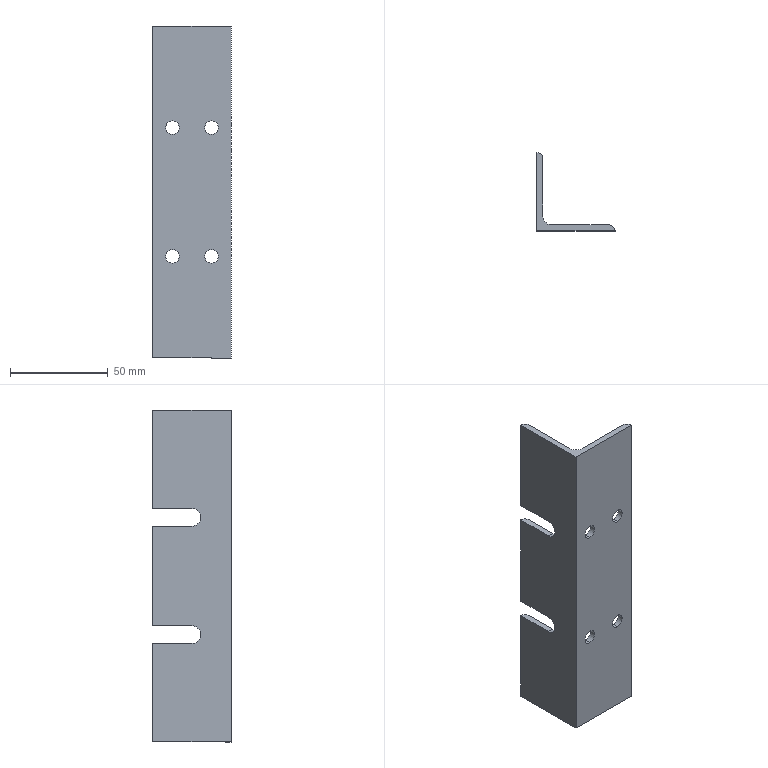Part | SolidWorks | features BaseBody 1 | 1 solid | 25 faces | box 40 x 40 x 170 mm | volume 37654 mm3 | cylinder 15 | plane 10 | commonest cylinder face diameters 7 x8 6 x4 9 x3
STEP:
#1=CARTESIAN_POINT('',(30.,3.,-29.45));
#2=VERTEX_POINT('',#1);
#3=CARTESIAN_POINT('',(30.,0.,-29.45));
#4=VERTEX_POINT('',#3);
#5=CARTESIAN_POINT('',(30.,10.,-29.45));
#6=DIRECTION('',(0.,-1.,0.));
#7=VECTOR('',#6,1000.);
#8=LINE('',#5,#7);
#9=EDGE_CURVE('',#2,#4,#8,.T.);
#10=ORIENTED_EDGE('',*,*,#9,.F.);
#11=CARTESIAN_POINT('',(30.,3.,-36.45));
#12=VERTEX_POINT('',#11);
#13=CARTESIAN_POINT('',(30.,3.,-32.95));
#14=DIRECTION('',(0.,-1.,0.));
#15=DIRECTION('',(0.,0.,-1.));
#16=AXIS2_PLACEMENT_3D('',#13,#14,#15);
#17=CIRCLE('',#16,3.5);
#18=EDGE_CURVE('',#12,#2,#17,.T.);
#19=ORIENTED_EDGE('',*,*,#18,.F.);
#20=CARTESIAN_POINT('',(30.,0.,-36.45));
#21=VERTEX_POINT('',#20);
#22=CARTESIAN_POINT('',(30.,10.,-36.45));
#23=DIRECTION('',(0.,-1.,0.));
#24=VECTOR('',#23,1000.);
#25=LINE('',#22,#24);
#26=EDGE_CURVE('',#12,#21,#25,.T.);
#27=ORIENTED_EDGE('',*,*,#26,.T.);
#28=CARTESIAN_POINT('',(30.,0.,-32.95));
#29=DIRECTION('',(0.,-1.,0.));
#30=DIRECTION('',(0.,0.,1.));
#31=AXIS2_PLACEMENT_3D('',#28,#29,#30);
#32=CIRCLE('',#31,3.5);
#33=EDGE_CURVE('',#21,#4,#32,.T.);
#34=ORIENTED_EDGE('',*,*,#33,.T.);
#35=EDGE_LOOP('',(#10,#19,#27,#34));
#36=FACE_OUTER_BOUND('',#35,.T.);
#37=CARTESIAN_POINT('',(30.,10.,-32.95));
#38=DIRECTION('',(0.,-1.,0.));
#39=DIRECTION('',(0.,0.,-1.));
#40=AXIS2_PLACEMENT_3D('',#37,#38,#39);
#41=CYLINDRICAL_SURFACE('',#40,3.5);
#42=ADVANCED_FACE('',(#36),#41,.F.);
#43=CARTESIAN_POINT('',(30.,3.,36.45));
#44=VERTEX_POINT('',#43);
#45=CARTESIAN_POINT('',(30.,0.,36.45));
#46=VERTEX_POINT('',#45);
#47=CARTESIAN_POINT('',(30.,10.,36.45));
#48=DIRECTION('',(0.,-1.,0.));
#49=VECTOR('',#48,1000.);
#50=LINE('',#47,#49);
#51=EDGE_CURVE('',#44,#46,#50,.T.);
#52=ORIENTED_EDGE('',*,*,#51,.F.);
#53=CARTESIAN_POINT('',(30.,3.,29.45));
#54=VERTEX_POINT('',#53);
#55=CARTESIAN_POINT('',(30.,3.,32.95));
#56=DIRECTION('',(0.,-1.,0.));
#57=DIRECTION('',(0.,0.,-1.));
#58=AXIS2_PLACEMENT_3D('',#55,#56,#57);
#59=CIRCLE('',#58,3.5);
#60=EDGE_CURVE('',#54,#44,#59,.T.);
#61=ORIENTED_EDGE('',*,*,#60,.F.);
#62=CARTESIAN_POINT('',(30.,0.,29.45));
#63=VERTEX_POINT('',#62);
#64=CARTESIAN_POINT('',(30.,10.,29.45));
#65=DIRECTION('',(0.,-1.,0.));
#66=VECTOR('',#65,1000.);
#67=LINE('',#64,#66);
#68=EDGE_CURVE('',#54,#63,#67,.T.);
#69=ORIENTED_EDGE('',*,*,#68,.T.);
#70=CARTESIAN_POINT('',(30.,0.,32.95));
#71=DIRECTION('',(0.,-1.,0.));
#72=DIRECTION('',(0.,0.,-1.));
#73=AXIS2_PLACEMENT_3D('',#70,#71,#72);
#74=CIRCLE('',#73,3.5);
#75=EDGE_CURVE('',#63,#46,#74,.T.);
#76=ORIENTED_EDGE('',*,*,#75,.T.);
#77=EDGE_LOOP('',(#52,#61,#69,#76));
#78=FACE_OUTER_BOUND('',#77,.T.);
#79=CARTESIAN_POINT('',(30.,10.,32.95));
#80=DIRECTION('',(0.,-1.,0.));
#81=DIRECTION('',(0.,0.,-1.));
#82=AXIS2_PLACEMENT_3D('',#79,#80,#81);
#83=CYLINDRICAL_SURFACE('',#82,3.5);
#84=ADVANCED_FACE('',(#78),#83,.F.);
#85=CARTESIAN_POINT('',(10.,3.,-29.45));
#86=VERTEX_POINT('',#85);
#87=CARTESIAN_POINT('',(10.,0.,-29.45));
#88=VERTEX_POINT('',#87);
#89=CARTESIAN_POINT('',(10.,10.,-29.45));
#90=DIRECTION('',(0.,-1.,0.));
#91=VECTOR('',#90,1000.);
#92=LINE('',#89,#91);
#93=EDGE_CURVE('',#86,#88,#92,.T.);
#94=ORIENTED_EDGE('',*,*,#93,.F.);
#95=CARTESIAN_POINT('',(10.,3.,-36.45));
#96=VERTEX_POINT('',#95);
#97=CARTESIAN_POINT('',(10.,3.,-32.95));
#98=DIRECTION('',(0.,-1.,0.));
#99=DIRECTION('',(0.,0.,-1.));
#100=AXIS2_PLACEMENT_3D('',#97,#98,#99);
#101=CIRCLE('',#100,3.5);
#102=EDGE_CURVE('',#96,#86,#101,.T.);
#103=ORIENTED_EDGE('',*,*,#102,.F.);
#104=CARTESIAN_POINT('',(10.,0.,-36.45));
#105=VERTEX_POINT('',#104);
#106=CARTESIAN_POINT('',(10.,10.,-36.45));
#107=DIRECTION('',(0.,-1.,0.));
#108=VECTOR('',#107,1000.);
#109=LINE('',#106,#108);
#110=EDGE_CURVE('',#96,#105,#109,.T.);
#111=ORIENTED_EDGE('',*,*,#110,.T.);
#112=CARTESIAN_POINT('',(10.,0.,-32.95));
#113=DIRECTION('',(0.,-1.,0.));
#114=DIRECTION('',(0.,0.,1.));
#115=AXIS2_PLACEMENT_3D('',#112,#113,#114);
#116=CIRCLE('',#115,3.5);
#117=EDGE_CURVE('',#105,#88,#116,.T.);
#118=ORIENTED_EDGE('',*,*,#117,.T.);
#119=EDGE_LOOP('',(#94,#103,#111,#118));
#120=FACE_OUTER_BOUND('',#119,.T.);
#121=CARTESIAN_POINT('',(10.,10.,-32.95));
#122=DIRECTION('',(0.,-1.,0.));
#123=DIRECTION('',(0.,0.,-1.));
#124=AXIS2_PLACEMENT_3D('',#121,#122,#123);
#125=CYLINDRICAL_SURFACE('',#124,3.5);
#126=ADVANCED_FACE('',(#120),#125,.F.);
#127=CARTESIAN_POINT('',(10.,3.,36.45));
#128=VERTEX_POINT('',#127);
#129=CARTESIAN_POINT('',(10.,0.,36.45));
#130=VERTEX_POINT('',#129);
#131=CARTESIAN_POINT('',(10.,10.,36.45));
#132=DIRECTION('',(0.,-1.,0.));
#133=VECTOR('',#132,1000.);
#134=LINE('',#131,#133);
#135=EDGE_CURVE('',#128,#130,#134,.T.);
#136=ORIENTED_EDGE('',*,*,#135,.F.);
#137=CARTESIAN_POINT('',(10.,3.,29.45));
#138=VERTEX_POINT('',#137);
#139=CARTESIAN_POINT('',(10.,3.,32.95));
#140=DIRECTION('',(0.,-1.,0.));
#141=DIRECTION('',(0.,0.,-1.));
#142=AXIS2_PLACEMENT_3D('',#139,#140,#141);
#143=CIRCLE('',#142,3.5);
#144=EDGE_CURVE('',#138,#128,#143,.T.);
#145=ORIENTED_EDGE('',*,*,#144,.F.);
#146=CARTESIAN_POINT('',(10.,0.,29.45));
#147=VERTEX_POINT('',#146);
#148=CARTESIAN_POINT('',(10.,10.,29.45));
#149=DIRECTION('',(0.,-1.,0.));
#150=VECTOR('',#149,1000.);
#151=LINE('',#148,#150);
#152=EDGE_CURVE('',#138,#147,#151,.T.);
#153=ORIENTED_EDGE('',*,*,#152,.T.);
#154=CARTESIAN_POINT('',(10.,0.,32.95));
#155=DIRECTION('',(0.,-1.,0.));
#156=DIRECTION('',(0.,0.,-1.));
#157=AXIS2_PLACEMENT_3D('',#154,#155,#156);
#158=CIRCLE('',#157,3.5);
#159=EDGE_CURVE('',#147,#130,#158,.T.);
#160=ORIENTED_EDGE('',*,*,#159,.T.);
#161=EDGE_LOOP('',(#136,#145,#153,#160));
#162=FACE_OUTER_BOUND('',#161,.T.);
#163=CARTESIAN_POINT('',(10.,10.,32.95));
#164=DIRECTION('',(0.,-1.,0.));
#165=DIRECTION('',(0.,0.,-1.));
#166=AXIS2_PLACEMENT_3D('',#163,#164,#165);
#167=CYLINDRICAL_SURFACE('',#166,3.5);
#168=ADVANCED_FACE('',(#162),#167,.F.);
#169=CARTESIAN_POINT('',(3.,37.,25.5));
#170=VERTEX_POINT('',#169);
#171=CARTESIAN_POINT('',(0.,40.,25.5));
#172=VERTEX_POINT('',#171);
#173=CARTESIAN_POINT('',(0.,37.,25.5));
#174=DIRECTION('',(0.,0.,1.));
#175=DIRECTION('',(0.,1.,0.));
#176=AXIS2_PLACEMENT_3D('',#173,#174,#175);
#177=CIRCLE('',#176,3.);
#178=EDGE_CURVE('',#170,#172,#177,.T.);
#179=ORIENTED_EDGE('',*,*,#178,.T.);
#180=CARTESIAN_POINT('',(0.,20.,25.5));
#181=VERTEX_POINT('',#180);
#182=CARTESIAN_POINT('',(0.,40.,25.5));
#183=DIRECTION('',(0.,-1.,0.));
#184=VECTOR('',#183,1000.);
#185=LINE('',#182,#184);
#186=EDGE_CURVE('',#172,#181,#185,.T.);
#187=ORIENTED_EDGE('',*,*,#186,.T.);
#188=CARTESIAN_POINT('',(3.,20.,25.5));
#189=VERTEX_POINT('',#188);
#190=CARTESIAN_POINT('',(10.,20.,25.5));
#191=DIRECTION('',(-1.,0.,0.));
#192=VECTOR('',#191,1000.);
#193=LINE('',#190,#192);
#194=EDGE_CURVE('',#189,#181,#193,.T.);
#195=ORIENTED_EDGE('',*,*,#194,.F.);
#196=CARTESIAN_POINT('',(3.,40.,25.5));
#197=DIRECTION('',(0.,-1.,0.));
#198=VECTOR('',#197,1000.);
#199=LINE('',#196,#198);
#200=EDGE_CURVE('',#170,#189,#199,.T.);
#201=ORIENTED_EDGE('',*,*,#200,.F.);
#202=EDGE_LOOP('',(#179,#187,#195,#201));
#203=FACE_OUTER_BOUND('',#202,.T.);
#204=CARTESIAN_POINT('',(10.,40.,25.5));
#205=DIRECTION('',(0.,0.,-1.));
#206=DIRECTION('',(0.,-1.,0.));
#207=AXIS2_PLACEMENT_3D('',#204,#205,#206);
#208=PLANE('',#207);
#209=ADVANCED_FACE('',(#203),#208,.F.);
#210=CARTESIAN_POINT('',(3.,20.,34.5));
#211=VERTEX_POINT('',#210);
#212=CARTESIAN_POINT('',(0.,20.,34.5));
#213=VERTEX_POINT('',#212);
#214=CARTESIAN_POINT('',(10.,20.,34.5));
#215=DIRECTION('',(-1.,0.,0.));
#216=VECTOR('',#215,1000.);
#217=LINE('',#214,#216);
#218=EDGE_CURVE('',#211,#213,#217,.T.);
#219=ORIENTED_EDGE('',*,*,#218,.T.);
#220=CARTESIAN_POINT('',(0.,40.,34.5));
#221=VERTEX_POINT('',#220);
#222=CARTESIAN_POINT('',(0.,40.,34.5));
#223=DIRECTION('',(0.,1.,0.));
#224=VECTOR('',#223,1000.);
#225=LINE('',#222,#224);
#226=EDGE_CURVE('',#213,#221,#225,.T.);
#227=ORIENTED_EDGE('',*,*,#226,.T.);
#228=CARTESIAN_POINT('',(3.,37.,34.5));
#229=VERTEX_POINT('',#228);
#230=CARTESIAN_POINT('',(0.,37.,34.5));
#231=DIRECTION('',(0.,0.,-1.));
#232=DIRECTION('',(0.,-1.,0.));
#233=AXIS2_PLACEMENT_3D('',#230,#231,#232);
#234=CIRCLE('',#233,3.);
#235=EDGE_CURVE('',#221,#229,#234,.T.);
#236=ORIENTED_EDGE('',*,*,#235,.T.);
#237=CARTESIAN_POINT('',(3.,40.,34.5));
#238=DIRECTION('',(0.,1.,0.));
#239=VECTOR('',#238,1000.);
#240=LINE('',#237,#239);
#241=EDGE_CURVE('',#211,#229,#240,.T.);
#242=ORIENTED_EDGE('',*,*,#241,.F.);
#243=EDGE_LOOP('',(#219,#227,#236,#242));
#244=FACE_OUTER_BOUND('',#243,.T.);
#245=CARTESIAN_POINT('',(10.,40.,34.5));
#246=DIRECTION('',(0.,0.,1.));
#247=DIRECTION('',(0.,-1.,0.));
#248=AXIS2_PLACEMENT_3D('',#245,#246,#247);
#249=PLANE('',#248);
#250=ADVANCED_FACE('',(#244),#249,.F.);
#251=ORIENTED_EDGE('',*,*,#194,.T.);
#252=CARTESIAN_POINT('',(0.,20.,30.));
#253=DIRECTION('',(-1.,0.,0.));
#254=DIRECTION('',(0.,0.,1.));
#255=AXIS2_PLACEMENT_3D('',#252,#253,#254);
#256=CIRCLE('',#255,4.5);
#257=EDGE_CURVE('',#181,#213,#256,.T.);
#258=ORIENTED_EDGE('',*,*,#257,.T.);
#259=ORIENTED_EDGE('',*,*,#218,.F.);
#260=CARTESIAN_POINT('',(3.,20.,30.));
#261=DIRECTION('',(-1.,0.,0.));
#262=DIRECTION('',(0.,-1.,0.));
#263=AXIS2_PLACEMENT_3D('',#260,#261,#262);
#264=CIRCLE('',#263,4.5);
#265=EDGE_CURVE('',#189,#211,#264,.T.);
#266=ORIENTED_EDGE('',*,*,#265,.F.);
#267=EDGE_LOOP('',(#251,#258,#259,#266));
#268=FACE_OUTER_BOUND('',#267,.T.);
#269=CARTESIAN_POINT('',(10.,20.,30.));
#270=DIRECTION('',(-1.,0.,0.));
#271=DIRECTION('',(0.,0.,1.));
#272=AXIS2_PLACEMENT_3D('',#269,#270,#271);
#273=CYLINDRICAL_SURFACE('',#272,4.5);
#274=ADVANCED_FACE('',(#268),#273,.F.);
#275=CARTESIAN_POINT('',(3.,37.,-34.5));
#276=VERTEX_POINT('',#275);
#277=CARTESIAN_POINT('',(0.,40.,-34.5));
#278=VERTEX_POINT('',#277);
#279=CARTESIAN_POINT('',(0.,37.,-34.5));
#280=DIRECTION('',(0.,0.,1.));
#281=DIRECTION('',(0.,1.,0.));
#282=AXIS2_PLACEMENT_3D('',#279,#280,#281);
#283=CIRCLE('',#282,3.);
#284=EDGE_CURVE('',#276,#278,#283,.T.);
#285=ORIENTED_EDGE('',*,*,#284,.T.);
#286=CARTESIAN_POINT('',(0.,20.,-34.5));
#287=VERTEX_POINT('',#286);
#288=CARTESIAN_POINT('',(0.,40.,-34.5));
#289=DIRECTION('',(0.,-1.,0.));
#290=VECTOR('',#289,1000.);
#291=LINE('',#288,#290);
#292=EDGE_CURVE('',#278,#287,#291,.T.);
#293=ORIENTED_EDGE('',*,*,#292,.T.);
#294=CARTESIAN_POINT('',(3.,20.,-34.5));
#295=VERTEX_POINT('',#294);
#296=CARTESIAN_POINT('',(10.,20.,-34.5));
#297=DIRECTION('',(-1.,0.,0.));
#298=VECTOR('',#297,1000.);
#299=LINE('',#296,#298);
#300=EDGE_CURVE('',#295,#287,#299,.T.);
#301=ORIENTED_EDGE('',*,*,#300,.F.);
#302=CARTESIAN_POINT('',(3.,40.,-34.5));
#303=DIRECTION('',(0.,-1.,0.));
#304=VECTOR('',#303,1000.);
#305=LINE('',#302,#304);
#306=EDGE_CURVE('',#276,#295,#305,.T.);
#307=ORIENTED_EDGE('',*,*,#306,.F.);
#308=EDGE_LOOP('',(#285,#293,#301,#307));
#309=FACE_OUTER_BOUND('',#308,.T.);
#310=CARTESIAN_POINT('',(10.,40.,-34.5));
#311=DIRECTION('',(0.,0.,-1.));
#312=DIRECTION('',(0.,-1.,0.));
#313=AXIS2_PLACEMENT_3D('',#310,#311,#312);
#314=PLANE('',#313);
#315=ADVANCED_FACE('',(#309),#314,.F.);
#316=CARTESIAN_POINT('',(3.,20.,-25.5));
#317=VERTEX_POINT('',#316);
#318=CARTESIAN_POINT('',(0.,20.,-25.5));
#319=VERTEX_POINT('',#318);
#320=CARTESIAN_POINT('',(10.,20.,-25.5));
#321=DIRECTION('',(-1.,0.,0.));
#322=VECTOR('',#321,1000.);
#323=LINE('',#320,#322);
#324=EDGE_CURVE('',#317,#319,#323,.T.);
#325=ORIENTED_EDGE('',*,*,#324,.T.);
#326=CARTESIAN_POINT('',(0.,40.,-25.5));
#327=VERTEX_POINT('',#326);
#328=CARTESIAN_POINT('',(0.,40.,-25.5));
#329=DIRECTION('',(0.,1.,0.));
#330=VECTOR('',#329,1000.);
#331=LINE('',#328,#330);
#332=EDGE_CURVE('',#319,#327,#331,.T.);
#333=ORIENTED_EDGE('',*,*,#332,.T.);
#334=CARTESIAN_POINT('',(3.,37.,-25.5));
#335=VERTEX_POINT('',#334);
#336=CARTESIAN_POINT('',(0.,37.,-25.5));
#337=DIRECTION('',(0.,0.,-1.));
#338=DIRECTION('',(1.,0.,0.));
#339=AXIS2_PLACEMENT_3D('',#336,#337,#338);
#340=CIRCLE('',#339,3.);
#341=EDGE_CURVE('',#327,#335,#340,.T.);
#342=ORIENTED_EDGE('',*,*,#341,.T.);
#343=CARTESIAN_POINT('',(3.,40.,-25.5));
#344=DIRECTION('',(0.,1.,0.));
#345=VECTOR('',#344,1000.);
#346=LINE('',#343,#345);
#347=EDGE_CURVE('',#317,#335,#346,.T.);
#348=ORIENTED_EDGE('',*,*,#347,.F.);
#349=EDGE_LOOP('',(#325,#333,#342,#348));
#350=FACE_OUTER_BOUND('',#349,.T.);
#351=CARTESIAN_POINT('',(10.,40.,-25.5));
#352=DIRECTION('',(0.,0.,1.));
#353=DIRECTION('',(1.,0.,0.));
#354=AXIS2_PLACEMENT_3D('',#351,#352,#353);
#355=PLANE('',#354);
#356=ADVANCED_FACE('',(#350),#355,.F.);
#357=ORIENTED_EDGE('',*,*,#300,.T.);
#358=CARTESIAN_POINT('',(0.,20.,-30.));
#359=DIRECTION('',(-1.,0.,0.));
#360=DIRECTION('',(0.,0.,-1.));
#361=AXIS2_PLACEMENT_3D('',#358,#359,#360);
#362=CIRCLE('',#361,4.5);
#363=EDGE_CURVE('',#287,#319,#362,.T.);
#364=ORIENTED_EDGE('',*,*,#363,.T.);
#365=ORIENTED_EDGE('',*,*,#324,.F.);
#366=CARTESIAN_POINT('',(3.,20.,-30.));
#367=DIRECTION('',(-1.,0.,0.));
#368=DIRECTION('',(0.,-1.,0.));
#369=AXIS2_PLACEMENT_3D('',#366,#367,#368);
#370=CIRCLE('',#369,4.5);
#371=EDGE_CURVE('',#295,#317,#370,.T.);
#372=ORIENTED_EDGE('',*,*,#371,.F.);
#373=EDGE_LOOP('',(#357,#364,#365,#372));
#374=FACE_OUTER_BOUND('',#373,.T.);
#375=CARTESIAN_POINT('',(10.,20.,-30.));
#376=DIRECTION('',(-1.,0.,0.));
#377=DIRECTION('',(0.,0.,1.));
#378=AXIS2_PLACEMENT_3D('',#375,#376,#377);
#379=CYLINDRICAL_SURFACE('',#378,4.5);
#380=ADVANCED_FACE('',(#374),#379,.F.);
#381=ORIENTED_EDGE('',*,*,#284,.F.);
#382=CARTESIAN_POINT('',(3.,37.,-85.));
#383=VERTEX_POINT('',#382);
#384=CARTESIAN_POINT('',(3.,37.,85.));
#385=DIRECTION('',(0.,0.,1.));
#386=VECTOR('',#385,1000.);
#387=LINE('',#384,#386);
#388=EDGE_CURVE('',#383,#276,#387,.T.);
#389=ORIENTED_EDGE('',*,*,#388,.F.);
#390=CARTESIAN_POINT('',(0.,40.,-85.));
#391=VERTEX_POINT('',#390);
#392=CARTESIAN_POINT('',(0.,37.,-85.));
#393=DIRECTION('',(0.,0.,-1.));
#394=DIRECTION('',(-1.,0.,0.));
#395=AXIS2_PLACEMENT_3D('',#392,#393,#394);
#396=CIRCLE('',#395,3.);
#397=EDGE_CURVE('',#391,#383,#396,.T.);
#398=ORIENTED_EDGE('',*,*,#397,.F.);
#399=CARTESIAN_POINT('',(0.,40.,85.));
#400=DIRECTION('',(0.,0.,-1.));
#401=VECTOR('',#400,1000.);
#402=LINE('',#399,#401);
#403=EDGE_CURVE('',#278,#391,#402,.T.);
#404=ORIENTED_EDGE('',*,*,#403,.F.);
#405=EDGE_LOOP('',(#381,#389,#398,#404));
#406=FACE_OUTER_BOUND('',#405,.T.);
#407=CARTESIAN_POINT('',(0.,37.,85.));
#408=DIRECTION('',(0.,0.,-1.));
#409=DIRECTION('',(-1.,0.,0.));
#410=AXIS2_PLACEMENT_3D('',#407,#408,#409);
#411=CYLINDRICAL_SURFACE('',#410,3.);
#412=ADVANCED_FACE('',(#406),#411,.T.);
#413=CARTESIAN_POINT('',(40.,0.,85.));
#414=VERTEX_POINT('',#413);
#415=CARTESIAN_POINT('',(37.,3.,85.));
#416=VERTEX_POINT('',#415);
#417=CARTESIAN_POINT('',(37.,0.,85.));
#418=DIRECTION('',(0.,0.,1.));
#419=DIRECTION('',(-1.,0.,0.));
#420=AXIS2_PLACEMENT_3D('',#417,#418,#419);
#421=CIRCLE('',#420,3.);
#422=EDGE_CURVE('',#414,#416,#421,.T.);
#423=ORIENTED_EDGE('',*,*,#422,.F.);
#424=CARTESIAN_POINT('',(40.,0.,-85.));
#425=VERTEX_POINT('',#424);
#426=CARTESIAN_POINT('',(40.,0.,85.));
#427=DIRECTION('',(0.,0.,-1.));
#428=VECTOR('',#427,1000.);
#429=LINE('',#426,#428);
#430=EDGE_CURVE('',#414,#425,#429,.T.);
#431=ORIENTED_EDGE('',*,*,#430,.T.);
#432=CARTESIAN_POINT('',(37.,3.,-85.));
#433=VERTEX_POINT('',#432);
#434=CARTESIAN_POINT('',(37.,0.,-85.));
#435=DIRECTION('',(0.,0.,-1.));
#436=DIRECTION('',(-1.,0.,0.));
#437=AXIS2_PLACEMENT_3D('',#434,#435,#436);
#438=CIRCLE('',#437,3.);
#439=EDGE_CURVE('',#433,#425,#438,.T.);
#440=ORIENTED_EDGE('',*,*,#439,.F.);
#441=CARTESIAN_POINT('',(37.,3.,85.));
#442=DIRECTION('',(0.,0.,-1.));
#443=VECTOR('',#442,1000.);
#444=LINE('',#441,#443);
#445=EDGE_CURVE('',#416,#433,#444,.T.);
#446=ORIENTED_EDGE('',*,*,#445,.F.);
#447=EDGE_LOOP('',(#423,#431,#440,#446));
#448=FACE_OUTER_BOUND('',#447,.T.);
#449=CARTESIAN_POINT('',(37.,0.,85.));
#450=DIRECTION('',(0.,0.,-1.));
#451=DIRECTION('',(-1.,0.,0.));
#452=AXIS2_PLACEMENT_3D('',#449,#450,#451);
#453=CYLINDRICAL_SURFACE('',#452,3.);
#454=ADVANCED_FACE('',(#448),#453,.T.);
#455=CARTESIAN_POINT('',(7.5,3.,-30.501));
#456=VERTEX_POINT('',#455);
#457=CARTESIAN_POINT('',(7.5,3.,30.501));
#458=VERTEX_POINT('',#457);
#459=CARTESIAN_POINT('',(7.5,3.,85.));
#460=DIRECTION('',(0.,0.,1.));
#461=VECTOR('',#460,1000.);
#462=LINE('',#459,#461);
#463=EDGE_CURVE('',#456,#458,#462,.T.);
#464=ORIENTED_EDGE('',*,*,#463,.F.);
#465=CARTESIAN_POINT('',(7.5,3.,-35.399));
#466=VERTEX_POINT('',#465);
#467=CARTESIAN_POINT('',(7.5,3.,-30.501));
#468=CARTESIAN_POINT('',(7.183,3.,-30.824));
#469=CARTESIAN_POINT('',(6.93,3.033,-31.209));
#470=CARTESIAN_POINT('',(6.673,3.076,-31.84));
#471=CARTESIAN_POINT('',(6.609,3.089,-32.053));
#472=CARTESIAN_POINT('',(6.522,3.107,-32.5));
#473=CARTESIAN_POINT('',(6.5,3.113,-32.726));
#474=CARTESIAN_POINT('',(6.5,3.112,-33.405));
#475=CARTESIAN_POINT('',(6.589,3.09,-33.854));
#476=CARTESIAN_POINT('',(6.932,3.033,-34.694));
#477=CARTESIAN_POINT('',(7.184,3.,-35.077));
#478=CARTESIAN_POINT('',(7.5,3.,-35.399));
#479=B_SPLINE_CURVE_WITH_KNOTS('',3,(#467,#468,#469,#470,#471,#472,#473,#474,#475,#476,#477,#478),.UNSPECIFIED.,.F.,.F.,(4,2,2,2,2,4),(0.,0.25,0.375,0.5,0.75,1.),.UNSPECIFIED.);
#480=EDGE_CURVE('',#456,#466,#479,.T.);
#481=ORIENTED_EDGE('',*,*,#480,.T.);
#482=CARTESIAN_POINT('',(7.5,3.,-85.));
#483=VERTEX_POINT('',#482);
#484=CARTESIAN_POINT('',(7.5,3.,85.));
#485=DIRECTION('',(0.,0.,1.));
#486=VECTOR('',#485,1000.);
#487=LINE('',#484,#486);
#488=EDGE_CURVE('',#483,#466,#487,.T.);
#489=ORIENTED_EDGE('',*,*,#488,.F.);
#490=CARTESIAN_POINT('',(3.,7.5,-85.));
#491=VERTEX_POINT('',#490);
#492=CARTESIAN_POINT('',(7.5,7.5,-85.));
#493=DIRECTION('',(0.,0.,1.));
#494=DIRECTION('',(-1.,0.,0.));
#495=AXIS2_PLACEMENT_3D('',#492,#493,#494);
#496=CIRCLE('',#495,4.5);
#497=EDGE_CURVE('',#491,#483,#496,.T.);
#498=ORIENTED_EDGE('',*,*,#497,.F.);
#499=CARTESIAN_POINT('',(3.,7.5,85.));
#500=VERTEX_POINT('',#499);
#501=CARTESIAN_POINT('',(3.,7.5,-85.));
#502=DIRECTION('',(0.,0.,-1.));
#503=VECTOR('',#502,1000.);
#504=LINE('',#501,#503);
#505=EDGE_CURVE('',#500,#491,#504,.T.);
#506=ORIENTED_EDGE('',*,*,#505,.F.);
#507=CARTESIAN_POINT('',(7.5,3.,85.));
#508=VERTEX_POINT('',#507);
#509=CARTESIAN_POINT('',(7.5,7.5,85.));
#510=DIRECTION('',(0.,0.,-1.));
#511=DIRECTION('',(-1.,0.,0.));
#512=AXIS2_PLACEMENT_3D('',#509,#510,#511);
#513=CIRCLE('',#512,4.5);
#514=EDGE_CURVE('',#508,#500,#513,.T.);
#515=ORIENTED_EDGE('',*,*,#514,.F.);
#516=CARTESIAN_POINT('',(7.5,3.,35.399));
#517=VERTEX_POINT('',#516);
#518=CARTESIAN_POINT('',(7.5,3.,85.));
#519=DIRECTION('',(0.,0.,1.));
#520=VECTOR('',#519,1000.);
#521=LINE('',#518,#520);
#522=EDGE_CURVE('',#517,#508,#521,.T.);
#523=ORIENTED_EDGE('',*,*,#522,.F.);
#524=CARTESIAN_POINT('',(7.5,3.,35.399));
#525=CARTESIAN_POINT('',(7.183,3.,35.076));
#526=CARTESIAN_POINT('',(6.93,3.033,34.691));
#527=CARTESIAN_POINT('',(6.673,3.076,34.06));
#528=CARTESIAN_POINT('',(6.609,3.089,33.847));
#529=CARTESIAN_POINT('',(6.522,3.107,33.4));
#530=CARTESIAN_POINT('',(6.5,3.113,33.174));
#531=CARTESIAN_POINT('',(6.5,3.112,32.495));
#532=CARTESIAN_POINT('',(6.589,3.09,32.046));
#533=CARTESIAN_POINT('',(6.932,3.033,31.206));
#534=CARTESIAN_POINT('',(7.184,3.,30.823));
#535=CARTESIAN_POINT('',(7.5,3.,30.501));
#536=B_SPLINE_CURVE_WITH_KNOTS('',3,(#524,#525,#526,#527,#528,#529,#530,#531,#532,#533,#534,#535),.UNSPECIFIED.,.F.,.F.,(4,2,2,2,2,4),(0.,0.25,0.375,0.5,0.75,1.),.UNSPECIFIED.);
#537=EDGE_CURVE('',#517,#458,#536,.T.);
#538=ORIENTED_EDGE('',*,*,#537,.T.);
#539=EDGE_LOOP('',(#464,#481,#489,#498,#506,#515,#523,#538));
#540=FACE_OUTER_BOUND('',#539,.T.);
#541=CARTESIAN_POINT('',(7.5,7.5,85.));
#542=DIRECTION('',(0.,0.,1.));
#543=DIRECTION('',(1.,0.,0.));
#544=AXIS2_PLACEMENT_3D('',#541,#542,#543);
#545=CYLINDRICAL_SURFACE('',#544,4.5);
#546=ADVANCED_FACE('',(#540),#545,.F.);
#547=CARTESIAN_POINT('',(3.,3.,-85.));
#548=DIRECTION('',(-1.,0.,0.));
#549=VECTOR('',#548,1000.);
#550=LINE('',#547,#549);
#551=EDGE_CURVE('',#433,#483,#550,.T.);
#552=ORIENTED_EDGE('',*,*,#551,.F.);
#553=ORIENTED_EDGE('',*,*,#439,.T.);
#554=CARTESIAN_POINT('',(0.,0.,-85.));
#555=VERTEX_POINT('',#554);
#556=CARTESIAN_POINT('',(0.,0.,-85.));
#557=DIRECTION('',(1.,0.,0.));
#558=VECTOR('',#557,1000.);
#559=LINE('',#556,#558);
#560=EDGE_CURVE('',#555,#425,#559,.T.);
#561=ORIENTED_EDGE('',*,*,#560,.F.);
#562=CARTESIAN_POINT('',(0.,0.,-85.));
#563=DIRECTION('',(0.,-1.,0.));
#564=VECTOR('',#563,1000.);
#565=LINE('',#562,#564);
#566=EDGE_CURVE('',#391,#555,#565,.T.);
#567=ORIENTED_EDGE('',*,*,#566,.F.);
#568=ORIENTED_EDGE('',*,*,#397,.T.);
#569=CARTESIAN_POINT('',(3.,40.,-85.));
#570=DIRECTION('',(0.,1.,0.));
#571=VECTOR('',#570,1000.);
#572=LINE('',#569,#571);
#573=EDGE_CURVE('',#491,#383,#572,.T.);
#574=ORIENTED_EDGE('',*,*,#573,.F.);
#575=ORIENTED_EDGE('',*,*,#497,.T.);
#576=EDGE_LOOP('',(#552,#553,#561,#567,#568,#574,#575));
#577=FACE_OUTER_BOUND('',#576,.T.);
#578=CARTESIAN_POINT('',(0.,0.,-85.));
#579=DIRECTION('',(0.,0.,-1.));
#580=DIRECTION('',(0.,-1.,0.));
#581=AXIS2_PLACEMENT_3D('',#578,#579,#580);
#582=PLANE('',#581);
#583=ADVANCED_FACE('',(#577),#582,.T.);
#584=CARTESIAN_POINT('',(0.,0.,85.));
#585=VERTEX_POINT('',#584);
#586=CARTESIAN_POINT('',(0.,0.,85.));
#587=DIRECTION('',(1.,0.,0.));
#588=VECTOR('',#587,1000.);
#589=LINE('',#586,#588);
#590=EDGE_CURVE('',#585,#414,#589,.T.);
#591=ORIENTED_EDGE('',*,*,#590,.T.);
#592=ORIENTED_EDGE('',*,*,#422,.T.);
#593=CARTESIAN_POINT('',(3.,3.,85.));
#594=DIRECTION('',(-1.,0.,0.));
#595=VECTOR('',#594,1000.);
#596=LINE('',#593,#595);
#597=EDGE_CURVE('',#416,#508,#596,.T.);
#598=ORIENTED_EDGE('',*,*,#597,.T.);
#599=ORIENTED_EDGE('',*,*,#514,.T.);
#600=CARTESIAN_POINT('',(3.,37.,85.));
#601=VERTEX_POINT('',#600);
#602=CARTESIAN_POINT('',(3.,40.,85.));
#603=DIRECTION('',(0.,1.,0.));
#604=VECTOR('',#603,1000.);
#605=LINE('',#602,#604);
#606=EDGE_CURVE('',#500,#601,#605,.T.);
#607=ORIENTED_EDGE('',*,*,#606,.T.);
#608=CARTESIAN_POINT('',(0.,40.,85.));
#609=VERTEX_POINT('',#608);
#610=CARTESIAN_POINT('',(0.,37.,85.));
#611=DIRECTION('',(0.,0.,1.));
#612=DIRECTION('',(-1.,0.,0.));
#613=AXIS2_PLACEMENT_3D('',#610,#611,#612);
#614=CIRCLE('',#613,3.);
#615=EDGE_CURVE('',#601,#609,#614,.T.);
#616=ORIENTED_EDGE('',*,*,#615,.T.);
#617=CARTESIAN_POINT('',(0.,0.,85.));
#618=DIRECTION('',(0.,-1.,0.));
#619=VECTOR('',#618,1000.);
#620=LINE('',#617,#619);
#621=EDGE_CURVE('',#609,#585,#620,.T.);
#622=ORIENTED_EDGE('',*,*,#621,.T.);
#623=EDGE_LOOP('',(#591,#592,#598,#599,#607,#616,#622));
#624=FACE_OUTER_BOUND('',#623,.T.);
#625=CARTESIAN_POINT('',(0.,0.,85.));
#626=DIRECTION('',(0.,0.,-1.));
#627=DIRECTION('',(0.,-1.,0.));
#628=AXIS2_PLACEMENT_3D('',#625,#626,#627);
#629=PLANE('',#628);
#630=ADVANCED_FACE('',(#624),#629,.F.);
#631=ORIENTED_EDGE('',*,*,#265,.T.);
#632=ORIENTED_EDGE('',*,*,#241,.T.);
#633=CARTESIAN_POINT('',(3.,37.,85.));
#634=DIRECTION('',(0.,0.,1.));
#635=VECTOR('',#634,1000.);
#636=LINE('',#633,#635);
#637=EDGE_CURVE('',#229,#601,#636,.T.);
#638=ORIENTED_EDGE('',*,*,#637,.T.);
#639=ORIENTED_EDGE('',*,*,#606,.F.);
#640=ORIENTED_EDGE('',*,*,#505,.T.);
#641=ORIENTED_EDGE('',*,*,#573,.T.);
#642=ORIENTED_EDGE('',*,*,#388,.T.);
#643=ORIENTED_EDGE('',*,*,#306,.T.);
#644=ORIENTED_EDGE('',*,*,#371,.T.);
#645=ORIENTED_EDGE('',*,*,#347,.T.);
#646=CARTESIAN_POINT('',(3.,37.,85.));
#647=DIRECTION('',(0.,0.,1.));
#648=VECTOR('',#647,1000.);
#649=LINE('',#646,#648);
#650=EDGE_CURVE('',#335,#170,#649,.T.);
#651=ORIENTED_EDGE('',*,*,#650,.T.);
#652=ORIENTED_EDGE('',*,*,#200,.T.);
#653=EDGE_LOOP('',(#631,#632,#638,#639,#640,#641,#642,#643,#644,#645,#651,#652));
#654=FACE_OUTER_BOUND('',#653,.T.);
#655=CARTESIAN_POINT('',(3.,40.,85.));
#656=DIRECTION('',(-1.,0.,0.));
#657=DIRECTION('',(0.,1.,0.));
#658=AXIS2_PLACEMENT_3D('',#655,#656,#657);
#659=PLANE('',#658);
#660=ADVANCED_FACE('',(#654),#659,.F.);
#661=ORIENTED_EDGE('',*,*,#60,.T.);
#662=CARTESIAN_POINT('',(30.,3.,32.95));
#663=DIRECTION('',(0.,-1.,0.));
#664=DIRECTION('',(0.,0.,-1.));
#665=AXIS2_PLACEMENT_3D('',#662,#663,#664);
#666=CIRCLE('',#665,3.5);
#667=EDGE_CURVE('',#44,#54,#666,.T.);
#668=ORIENTED_EDGE('',*,*,#667,.T.);
#669=EDGE_LOOP('',(#661,#668));
#670=FACE_BOUND('',#669,.T.);
#671=ORIENTED_EDGE('',*,*,#18,.T.);
#672=CARTESIAN_POINT('',(30.,3.,-32.95));
#673=DIRECTION('',(0.,-1.,0.));
#674=DIRECTION('',(0.,0.,-1.));
#675=AXIS2_PLACEMENT_3D('',#672,#673,#674);
#676=CIRCLE('',#675,3.5);
#677=EDGE_CURVE('',#2,#12,#676,.T.);
#678=ORIENTED_EDGE('',*,*,#677,.T.);
#679=EDGE_LOOP('',(#671,#678));
#680=FACE_BOUND('',#679,.T.);
#681=ORIENTED_EDGE('',*,*,#488,.T.);
#682=CARTESIAN_POINT('',(10.,3.,-32.95));
#683=DIRECTION('',(0.,-1.,0.));
#684=DIRECTION('',(0.,0.,-1.));
#685=AXIS2_PLACEMENT_3D('',#682,#683,#684);
#686=CIRCLE('',#685,3.5);
#687=EDGE_CURVE('',#466,#96,#686,.T.);
#688=ORIENTED_EDGE('',*,*,#687,.T.);
#689=ORIENTED_EDGE('',*,*,#102,.T.);
#690=CARTESIAN_POINT('',(10.,3.,-32.95));
#691=DIRECTION('',(0.,-1.,0.));
#692=DIRECTION('',(0.,0.,-1.));
#693=AXIS2_PLACEMENT_3D('',#690,#691,#692);
#694=CIRCLE('',#693,3.5);
#695=EDGE_CURVE('',#86,#456,#694,.T.);
#696=ORIENTED_EDGE('',*,*,#695,.T.);
#697=ORIENTED_EDGE('',*,*,#463,.T.);
#698=CARTESIAN_POINT('',(10.,3.,32.95));
#699=DIRECTION('',(0.,-1.,0.));
#700=DIRECTION('',(0.,0.,-1.));
#701=AXIS2_PLACEMENT_3D('',#698,#699,#700);
#702=CIRCLE('',#701,3.5);
#703=EDGE_CURVE('',#458,#138,#702,.T.);
#704=ORIENTED_EDGE('',*,*,#703,.T.);
#705=ORIENTED_EDGE('',*,*,#144,.T.);
#706=CARTESIAN_POINT('',(10.,3.,32.95));
#707=DIRECTION('',(0.,-1.,0.));
#708=DIRECTION('',(0.,0.,-1.));
#709=AXIS2_PLACEMENT_3D('',#706,#707,#708);
#710=CIRCLE('',#709,3.5);
#711=EDGE_CURVE('',#128,#517,#710,.T.);
#712=ORIENTED_EDGE('',*,*,#711,.T.);
#713=ORIENTED_EDGE('',*,*,#522,.T.);
#714=ORIENTED_EDGE('',*,*,#597,.F.);
#715=ORIENTED_EDGE('',*,*,#445,.T.);
#716=ORIENTED_EDGE('',*,*,#551,.T.);
#717=EDGE_LOOP('',(#681,#688,#689,#696,#697,#704,#705,#712,#713,#714,#715,#716));
#718=FACE_OUTER_BOUND('',#717,.T.);
#719=CARTESIAN_POINT('',(3.,3.,85.));
#720=DIRECTION('',(0.,-1.,0.));
#721=DIRECTION('',(0.,0.,-1.));
#722=AXIS2_PLACEMENT_3D('',#719,#720,#721);
#723=PLANE('',#722);
#724=ADVANCED_FACE('',(#670,#680,#718),#723,.F.);
#725=ORIENTED_EDGE('',*,*,#159,.F.);
#726=CARTESIAN_POINT('',(10.,0.,32.95));
#727=DIRECTION('',(0.,-1.,0.));
#728=DIRECTION('',(0.,0.,-1.));
#729=AXIS2_PLACEMENT_3D('',#726,#727,#728);
#730=CIRCLE('',#729,3.5);
#731=EDGE_CURVE('',#130,#147,#730,.T.);
#732=ORIENTED_EDGE('',*,*,#731,.F.);
#733=EDGE_LOOP('',(#725,#732));
#734=FACE_BOUND('',#733,.T.);
#735=ORIENTED_EDGE('',*,*,#75,.F.);
#736=CARTESIAN_POINT('',(30.,0.,32.95));
#737=DIRECTION('',(0.,-1.,0.));
#738=DIRECTION('',(0.,0.,-1.));
#739=AXIS2_PLACEMENT_3D('',#736,#737,#738);
#740=CIRCLE('',#739,3.5);
#741=EDGE_CURVE('',#46,#63,#740,.T.);
#742=ORIENTED_EDGE('',*,*,#741,.F.);
#743=EDGE_LOOP('',(#735,#742));
#744=FACE_BOUND('',#743,.T.);
#745=ORIENTED_EDGE('',*,*,#33,.F.);
#746=CARTESIAN_POINT('',(30.,0.,-32.95));
#747=DIRECTION('',(0.,-1.,0.));
#748=DIRECTION('',(0.,0.,1.));
#749=AXIS2_PLACEMENT_3D('',#746,#747,#748);
#750=CIRCLE('',#749,3.5);
#751=EDGE_CURVE('',#4,#21,#750,.T.);
#752=ORIENTED_EDGE('',*,*,#751,.F.);
#753=EDGE_LOOP('',(#745,#752));
#754=FACE_BOUND('',#753,.T.);
#755=ORIENTED_EDGE('',*,*,#117,.F.);
#756=CARTESIAN_POINT('',(10.,0.,-32.95));
#757=DIRECTION('',(0.,-1.,0.));
#758=DIRECTION('',(0.,0.,1.));
#759=AXIS2_PLACEMENT_3D('',#756,#757,#758);
#760=CIRCLE('',#759,3.5);
#761=EDGE_CURVE('',#88,#105,#760,.T.);
#762=ORIENTED_EDGE('',*,*,#761,.F.);
#763=EDGE_LOOP('',(#755,#762));
#764=FACE_BOUND('',#763,.T.);
#765=ORIENTED_EDGE('',*,*,#560,.T.);
#766=ORIENTED_EDGE('',*,*,#430,.F.);
#767=ORIENTED_EDGE('',*,*,#590,.F.);
#768=CARTESIAN_POINT('',(0.,0.,85.));
#769=DIRECTION('',(0.,0.,-1.));
#770=VECTOR('',#769,1000.);
#771=LINE('',#768,#770);
#772=EDGE_CURVE('',#585,#555,#771,.T.);
#773=ORIENTED_EDGE('',*,*,#772,.T.);
#774=EDGE_LOOP('',(#765,#766,#767,#773));
#775=FACE_OUTER_BOUND('',#774,.T.);
#776=CARTESIAN_POINT('',(0.,0.,85.));
#777=DIRECTION('',(0.,1.,0.));
#778=DIRECTION('',(1.,0.,0.));
#779=AXIS2_PLACEMENT_3D('',#776,#777,#778);
#780=PLANE('',#779);
#781=ADVANCED_FACE('',(#734,#744,#754,#764,#775),#780,.F.);
#782=CARTESIAN_POINT('',(0.,40.,85.));
#783=DIRECTION('',(0.,0.,-1.));
#784=VECTOR('',#783,1000.);
#785=LINE('',#782,#784);
#786=EDGE_CURVE('',#609,#221,#785,.T.);
#787=ORIENTED_EDGE('',*,*,#786,.T.);
#788=ORIENTED_EDGE('',*,*,#226,.F.);
#789=ORIENTED_EDGE('',*,*,#257,.F.);
#790=ORIENTED_EDGE('',*,*,#186,.F.);
#791=CARTESIAN_POINT('',(0.,40.,85.));
#792=DIRECTION('',(0.,0.,-1.));
#793=VECTOR('',#792,1000.);
#794=LINE('',#791,#793);
#795=EDGE_CURVE('',#172,#327,#794,.T.);
#796=ORIENTED_EDGE('',*,*,#795,.T.);
#797=ORIENTED_EDGE('',*,*,#332,.F.);
#798=ORIENTED_EDGE('',*,*,#363,.F.);
#799=ORIENTED_EDGE('',*,*,#292,.F.);
#800=ORIENTED_EDGE('',*,*,#403,.T.);
#801=ORIENTED_EDGE('',*,*,#566,.T.);
#802=ORIENTED_EDGE('',*,*,#772,.F.);
#803=ORIENTED_EDGE('',*,*,#621,.F.);
#804=EDGE_LOOP('',(#787,#788,#789,#790,#796,#797,#798,#799,#800,#801,#802,#803));
#805=FACE_OUTER_BOUND('',#804,.T.);
#806=CARTESIAN_POINT('',(0.,0.,85.));
#807=DIRECTION('',(1.,0.,0.));
#808=DIRECTION('',(0.,1.,0.));
#809=AXIS2_PLACEMENT_3D('',#806,#807,#808);
#810=PLANE('',#809);
#811=ADVANCED_FACE('',(#805),#810,.F.);
#812=ORIENTED_EDGE('',*,*,#178,.F.);
#813=ORIENTED_EDGE('',*,*,#650,.F.);
#814=ORIENTED_EDGE('',*,*,#341,.F.);
#815=ORIENTED_EDGE('',*,*,#795,.F.);
#816=EDGE_LOOP('',(#812,#813,#814,#815));
#817=FACE_OUTER_BOUND('',#816,.T.);
#818=CARTESIAN_POINT('',(0.,37.,85.));
#819=DIRECTION('',(0.,0.,-1.));
#820=DIRECTION('',(-1.,0.,0.));
#821=AXIS2_PLACEMENT_3D('',#818,#819,#820);
#822=CYLINDRICAL_SURFACE('',#821,3.);
#823=ADVANCED_FACE('',(#817),#822,.T.);
#824=ORIENTED_EDGE('',*,*,#235,.F.);
#825=ORIENTED_EDGE('',*,*,#786,.F.);
#826=ORIENTED_EDGE('',*,*,#615,.F.);
#827=ORIENTED_EDGE('',*,*,#637,.F.);
#828=EDGE_LOOP('',(#824,#825,#826,#827));
#829=FACE_OUTER_BOUND('',#828,.T.);
#830=CARTESIAN_POINT('',(0.,37.,85.));
#831=DIRECTION('',(0.,0.,-1.));
#832=DIRECTION('',(-1.,0.,0.));
#833=AXIS2_PLACEMENT_3D('',#830,#831,#832);
#834=CYLINDRICAL_SURFACE('',#833,3.);
#835=ADVANCED_FACE('',(#829),#834,.T.);
#836=ORIENTED_EDGE('',*,*,#711,.F.);
#837=ORIENTED_EDGE('',*,*,#135,.T.);
#838=ORIENTED_EDGE('',*,*,#731,.T.);
#839=ORIENTED_EDGE('',*,*,#152,.F.);
#840=ORIENTED_EDGE('',*,*,#703,.F.);
#841=ORIENTED_EDGE('',*,*,#537,.F.);
#842=EDGE_LOOP('',(#836,#837,#838,#839,#840,#841));
#843=FACE_OUTER_BOUND('',#842,.T.);
#844=CARTESIAN_POINT('',(10.,10.,32.95));
#845=DIRECTION('',(0.,-1.,0.));
#846=DIRECTION('',(0.,0.,-1.));
#847=AXIS2_PLACEMENT_3D('',#844,#845,#846);
#848=CYLINDRICAL_SURFACE('',#847,3.5);
#849=ADVANCED_FACE('',(#843),#848,.F.);
#850=ORIENTED_EDGE('',*,*,#695,.F.);
#851=ORIENTED_EDGE('',*,*,#93,.T.);
#852=ORIENTED_EDGE('',*,*,#761,.T.);
#853=ORIENTED_EDGE('',*,*,#110,.F.);
#854=ORIENTED_EDGE('',*,*,#687,.F.);
#855=ORIENTED_EDGE('',*,*,#480,.F.);
#856=EDGE_LOOP('',(#850,#851,#852,#853,#854,#855));
#857=FACE_OUTER_BOUND('',#856,.T.);
#858=CARTESIAN_POINT('',(10.,10.,-32.95));
#859=DIRECTION('',(0.,-1.,0.));
#860=DIRECTION('',(0.,0.,-1.));
#861=AXIS2_PLACEMENT_3D('',#858,#859,#860);
#862=CYLINDRICAL_SURFACE('',#861,3.5);
#863=ADVANCED_FACE('',(#857),#862,.F.);
#864=ORIENTED_EDGE('',*,*,#667,.F.);
#865=ORIENTED_EDGE('',*,*,#51,.T.);
#866=ORIENTED_EDGE('',*,*,#741,.T.);
#867=ORIENTED_EDGE('',*,*,#68,.F.);
#868=EDGE_LOOP('',(#864,#865,#866,#867));
#869=FACE_OUTER_BOUND('',#868,.T.);
#870=CARTESIAN_POINT('',(30.,10.,32.95));
#871=DIRECTION('',(0.,-1.,0.));
#872=DIRECTION('',(0.,0.,-1.));
#873=AXIS2_PLACEMENT_3D('',#870,#871,#872);
#874=CYLINDRICAL_SURFACE('',#873,3.5);
#875=ADVANCED_FACE('',(#869),#874,.F.);
#876=ORIENTED_EDGE('',*,*,#677,.F.);
#877=ORIENTED_EDGE('',*,*,#9,.T.);
#878=ORIENTED_EDGE('',*,*,#751,.T.);
#879=ORIENTED_EDGE('',*,*,#26,.F.);
#880=EDGE_LOOP('',(#876,#877,#878,#879));
#881=FACE_OUTER_BOUND('',#880,.T.);
#882=CARTESIAN_POINT('',(30.,10.,-32.95));
#883=DIRECTION('',(0.,-1.,0.));
#884=DIRECTION('',(0.,0.,-1.));
#885=AXIS2_PLACEMENT_3D('',#882,#883,#884);
#886=CYLINDRICAL_SURFACE('',#885,3.5);
#887=ADVANCED_FACE('',(#881),#886,.F.);
#888=CLOSED_SHELL('',(#42,#84,#126,#168,#209,#250,#274,#315,#356,#380,#412,#454,#546,#583,#630,#660,#724,#781,#811,#823,#835,#849,#863,#875,#887));
#889=MANIFOLD_SOLID_BREP('',#888);
#890=CARTESIAN_POINT('',(0.,0.,0.));
#891=DIRECTION('',(0.,0.,1.));
#892=DIRECTION('',(1.,0.,0.));
#893=AXIS2_PLACEMENT_3D('',#890,#891,#892);
#894=(LENGTH_UNIT()NAMED_UNIT(*)SI_UNIT(.MILLI.,.METRE.));
#895=UNCERTAINTY_MEASURE_WITH_UNIT(LENGTH_MEASURE(0.00001),#894,'','');
#896=(NAMED_UNIT(*)PLANE_ANGLE_UNIT()SI_UNIT($,.RADIAN.));
#897=(NAMED_UNIT(*)SI_UNIT($,.STERADIAN.)SOLID_ANGLE_UNIT());
#898=(GEOMETRIC_REPRESENTATION_CONTEXT(3)GLOBAL_UNCERTAINTY_ASSIGNED_CONTEXT((#895))GLOBAL_UNIT_ASSIGNED_CONTEXT((#894,#896,#897))REPRESENTATION_CONTEXT('',''));
#899=ADVANCED_BREP_SHAPE_REPRESENTATION('',(#889,#893),#898);